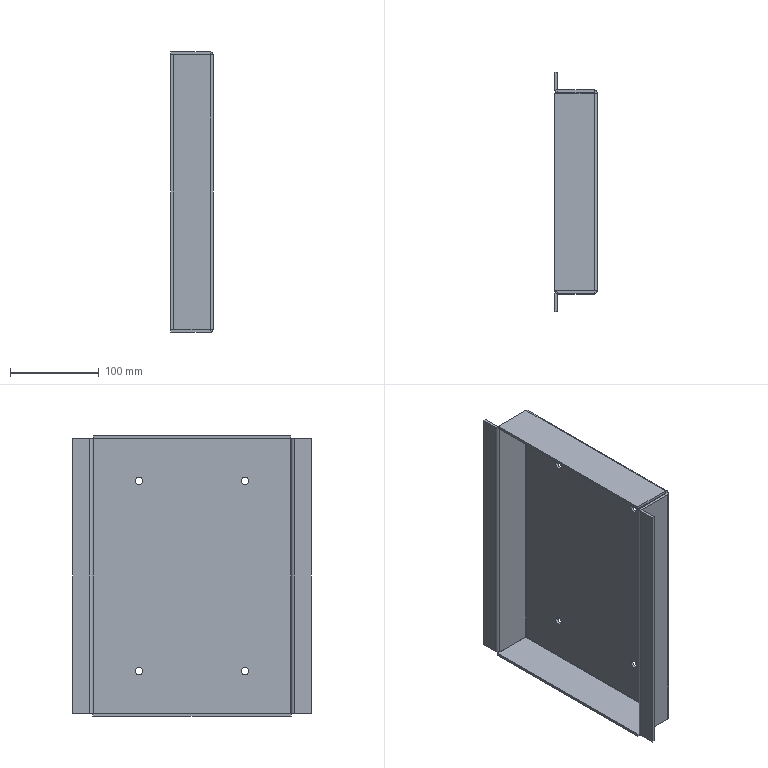Part | STEP file | SOLID | 1 solid | 64 faces | box 48 x 270 x 317 mm | volume 394936 mm3 | plane 40 | cylinder 20 | spline 4 | commonest cylinder face diameters 8.5 x8 1 x6 7 x6